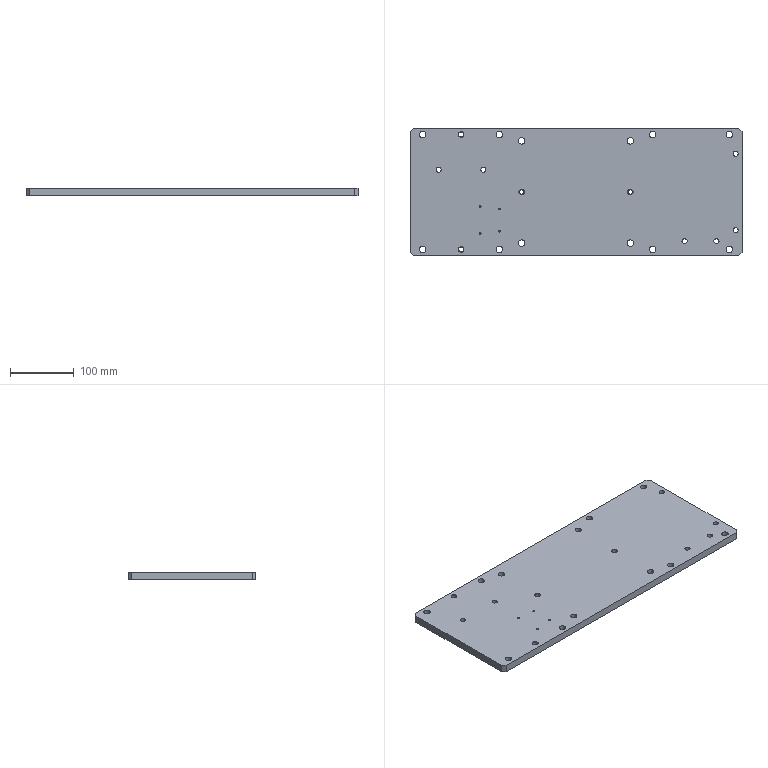Part | STEP file | J452-EBZ05-02-04-Part-1 | 1 solid | 82 faces | box 520 x 200 x 12 mm | volume 1229915 mm3 | cylinder 56 | plane 14 | cone 12 | commonest cylinder face diameters 10 x24 8 x20 2.5 x8 6.8 x4